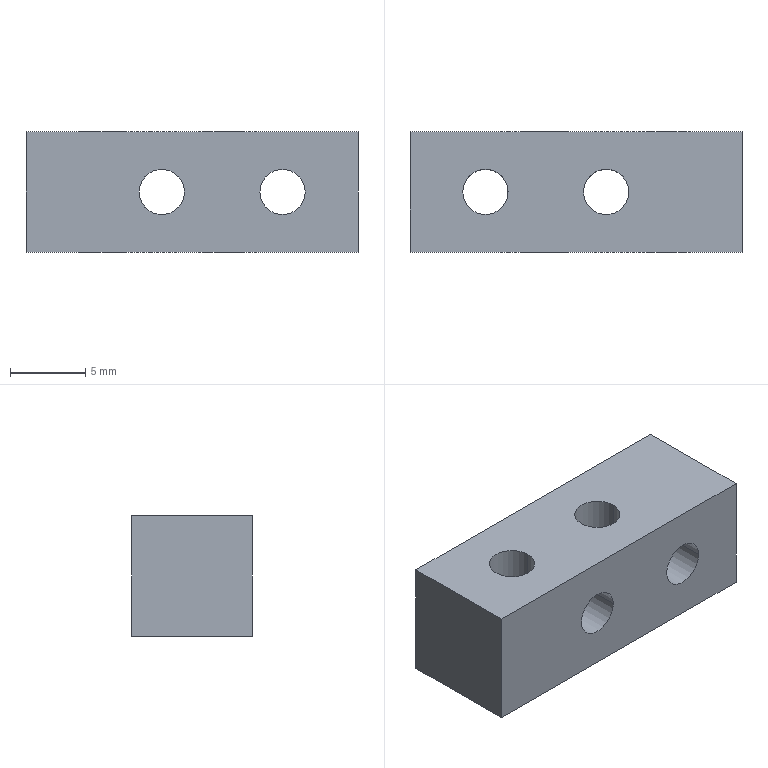Part | SolidWorks | features Extrusion 1, ICE 1 | 1 solid | 14 faces | box 22 x 8 x 8 mm | volume 1182 mm3 | cylinder 8 | plane 6 | commonest cylinder face diameters 3 x8
STEP:
#1=CARTESIAN_POINT('',(7.5,-4.,4.));
#2=VERTEX_POINT('',#1);
#3=CARTESIAN_POINT('',(4.5,-4.,4.));
#4=VERTEX_POINT('',#3);
#5=CARTESIAN_POINT('',(6.,-4.,4.));
#6=DIRECTION('',(0.,1.,0.));
#7=DIRECTION('',(-1.,0.,0.));
#8=AXIS2_PLACEMENT_3D('',#5,#6,#7);
#9=CIRCLE('',#8,1.5);
#10=EDGE_CURVE('',#2,#4,#9,.T.);
#11=ORIENTED_EDGE('',*,*,#10,.F.);
#12=CARTESIAN_POINT('',(7.5,4.,4.));
#13=VERTEX_POINT('',#12);
#14=CARTESIAN_POINT('',(7.5,-4.,4.));
#15=DIRECTION('',(0.,1.,0.));
#16=VECTOR('',#15,1000.);
#17=LINE('',#14,#16);
#18=EDGE_CURVE('',#2,#13,#17,.T.);
#19=ORIENTED_EDGE('',*,*,#18,.T.);
#20=CARTESIAN_POINT('',(4.5,4.,4.));
#21=VERTEX_POINT('',#20);
#22=CARTESIAN_POINT('',(6.,4.,4.));
#23=DIRECTION('',(0.,1.,0.));
#24=DIRECTION('',(-1.,0.,0.));
#25=AXIS2_PLACEMENT_3D('',#22,#23,#24);
#26=CIRCLE('',#25,1.5);
#27=EDGE_CURVE('',#13,#21,#26,.T.);
#28=ORIENTED_EDGE('',*,*,#27,.T.);
#29=CARTESIAN_POINT('',(4.5,-4.,4.));
#30=DIRECTION('',(0.,1.,0.));
#31=VECTOR('',#30,1000.);
#32=LINE('',#29,#31);
#33=EDGE_CURVE('',#4,#21,#32,.T.);
#34=ORIENTED_EDGE('',*,*,#33,.F.);
#35=EDGE_LOOP('',(#11,#19,#28,#34));
#36=FACE_OUTER_BOUND('',#35,.T.);
#37=CARTESIAN_POINT('',(6.,-4.,4.));
#38=DIRECTION('',(0.,1.,0.));
#39=DIRECTION('',(-1.,0.,0.));
#40=AXIS2_PLACEMENT_3D('',#37,#38,#39);
#41=CYLINDRICAL_SURFACE('',#40,1.5);
#42=ADVANCED_FACE('',(#36),#41,.F.);
#43=CARTESIAN_POINT('',(-0.5,-4.,4.));
#44=VERTEX_POINT('',#43);
#45=CARTESIAN_POINT('',(-3.5,-4.,4.));
#46=VERTEX_POINT('',#45);
#47=CARTESIAN_POINT('',(-2.,-4.,4.));
#48=DIRECTION('',(0.,1.,0.));
#49=DIRECTION('',(-1.,0.,0.));
#50=AXIS2_PLACEMENT_3D('',#47,#48,#49);
#51=CIRCLE('',#50,1.5);
#52=EDGE_CURVE('',#44,#46,#51,.T.);
#53=ORIENTED_EDGE('',*,*,#52,.F.);
#54=CARTESIAN_POINT('',(-0.5,4.,4.));
#55=VERTEX_POINT('',#54);
#56=CARTESIAN_POINT('',(-0.5,-4.,4.));
#57=DIRECTION('',(0.,1.,0.));
#58=VECTOR('',#57,1000.);
#59=LINE('',#56,#58);
#60=EDGE_CURVE('',#44,#55,#59,.T.);
#61=ORIENTED_EDGE('',*,*,#60,.T.);
#62=CARTESIAN_POINT('',(-3.5,4.,4.));
#63=VERTEX_POINT('',#62);
#64=CARTESIAN_POINT('',(-2.,4.,4.));
#65=DIRECTION('',(0.,1.,0.));
#66=DIRECTION('',(-1.,0.,0.));
#67=AXIS2_PLACEMENT_3D('',#64,#65,#66);
#68=CIRCLE('',#67,1.5);
#69=EDGE_CURVE('',#55,#63,#68,.T.);
#70=ORIENTED_EDGE('',*,*,#69,.T.);
#71=CARTESIAN_POINT('',(-3.5,-4.,4.));
#72=DIRECTION('',(0.,1.,0.));
#73=VECTOR('',#72,1000.);
#74=LINE('',#71,#73);
#75=EDGE_CURVE('',#46,#63,#74,.T.);
#76=ORIENTED_EDGE('',*,*,#75,.F.);
#77=EDGE_LOOP('',(#53,#61,#70,#76));
#78=FACE_OUTER_BOUND('',#77,.T.);
#79=CARTESIAN_POINT('',(-2.,-4.,4.));
#80=DIRECTION('',(0.,1.,0.));
#81=DIRECTION('',(-1.,0.,0.));
#82=AXIS2_PLACEMENT_3D('',#79,#80,#81);
#83=CYLINDRICAL_SURFACE('',#82,1.5);
#84=ADVANCED_FACE('',(#78),#83,.F.);
#85=CARTESIAN_POINT('',(0.5,0.,8.));
#86=VERTEX_POINT('',#85);
#87=CARTESIAN_POINT('',(3.5,0.,8.));
#88=VERTEX_POINT('',#87);
#89=CARTESIAN_POINT('',(2.,0.,8.));
#90=DIRECTION('',(0.,0.,1.));
#91=DIRECTION('',(1.,0.,0.));
#92=AXIS2_PLACEMENT_3D('',#89,#90,#91);
#93=CIRCLE('',#92,1.5);
#94=EDGE_CURVE('',#86,#88,#93,.T.);
#95=ORIENTED_EDGE('',*,*,#94,.T.);
#96=CARTESIAN_POINT('',(3.5,0.,0.));
#97=VERTEX_POINT('',#96);
#98=CARTESIAN_POINT('',(3.5,0.,8.));
#99=DIRECTION('',(0.,0.,-1.));
#100=VECTOR('',#99,1000.);
#101=LINE('',#98,#100);
#102=EDGE_CURVE('',#88,#97,#101,.T.);
#103=ORIENTED_EDGE('',*,*,#102,.T.);
#104=CARTESIAN_POINT('',(0.5,0.,0.));
#105=VERTEX_POINT('',#104);
#106=CARTESIAN_POINT('',(2.,0.,0.));
#107=DIRECTION('',(0.,0.,1.));
#108=DIRECTION('',(1.,0.,0.));
#109=AXIS2_PLACEMENT_3D('',#106,#107,#108);
#110=CIRCLE('',#109,1.5);
#111=EDGE_CURVE('',#105,#97,#110,.T.);
#112=ORIENTED_EDGE('',*,*,#111,.F.);
#113=CARTESIAN_POINT('',(0.5,0.,8.));
#114=DIRECTION('',(0.,0.,-1.));
#115=VECTOR('',#114,1000.);
#116=LINE('',#113,#115);
#117=EDGE_CURVE('',#86,#105,#116,.T.);
#118=ORIENTED_EDGE('',*,*,#117,.F.);
#119=EDGE_LOOP('',(#95,#103,#112,#118));
#120=FACE_OUTER_BOUND('',#119,.T.);
#121=CARTESIAN_POINT('',(2.,0.,8.));
#122=DIRECTION('',(0.,0.,-1.));
#123=DIRECTION('',(-1.,0.,0.));
#124=AXIS2_PLACEMENT_3D('',#121,#122,#123);
#125=CYLINDRICAL_SURFACE('',#124,1.5);
#126=ADVANCED_FACE('',(#120),#125,.F.);
#127=CARTESIAN_POINT('',(-7.5,0.,8.));
#128=VERTEX_POINT('',#127);
#129=CARTESIAN_POINT('',(-4.5,0.,8.));
#130=VERTEX_POINT('',#129);
#131=CARTESIAN_POINT('',(-6.,0.,8.));
#132=DIRECTION('',(0.,0.,1.));
#133=DIRECTION('',(1.,0.,0.));
#134=AXIS2_PLACEMENT_3D('',#131,#132,#133);
#135=CIRCLE('',#134,1.5);
#136=EDGE_CURVE('',#128,#130,#135,.T.);
#137=ORIENTED_EDGE('',*,*,#136,.T.);
#138=CARTESIAN_POINT('',(-4.5,0.,0.));
#139=VERTEX_POINT('',#138);
#140=CARTESIAN_POINT('',(-4.5,0.,8.));
#141=DIRECTION('',(0.,0.,-1.));
#142=VECTOR('',#141,1000.);
#143=LINE('',#140,#142);
#144=EDGE_CURVE('',#130,#139,#143,.T.);
#145=ORIENTED_EDGE('',*,*,#144,.T.);
#146=CARTESIAN_POINT('',(-7.5,0.,0.));
#147=VERTEX_POINT('',#146);
#148=CARTESIAN_POINT('',(-6.,0.,0.));
#149=DIRECTION('',(0.,0.,1.));
#150=DIRECTION('',(1.,0.,0.));
#151=AXIS2_PLACEMENT_3D('',#148,#149,#150);
#152=CIRCLE('',#151,1.5);
#153=EDGE_CURVE('',#147,#139,#152,.T.);
#154=ORIENTED_EDGE('',*,*,#153,.F.);
#155=CARTESIAN_POINT('',(-7.5,0.,8.));
#156=DIRECTION('',(0.,0.,-1.));
#157=VECTOR('',#156,1000.);
#158=LINE('',#155,#157);
#159=EDGE_CURVE('',#128,#147,#158,.T.);
#160=ORIENTED_EDGE('',*,*,#159,.F.);
#161=EDGE_LOOP('',(#137,#145,#154,#160));
#162=FACE_OUTER_BOUND('',#161,.T.);
#163=CARTESIAN_POINT('',(-6.,0.,8.));
#164=DIRECTION('',(0.,0.,-1.));
#165=DIRECTION('',(-1.,0.,0.));
#166=AXIS2_PLACEMENT_3D('',#163,#164,#165);
#167=CYLINDRICAL_SURFACE('',#166,1.5);
#168=ADVANCED_FACE('',(#162),#167,.F.);
#169=CARTESIAN_POINT('',(-11.,4.,8.));
#170=VERTEX_POINT('',#169);
#171=CARTESIAN_POINT('',(-11.,-4.,8.));
#172=VERTEX_POINT('',#171);
#173=CARTESIAN_POINT('',(-11.,4.,8.));
#174=DIRECTION('',(0.,-1.,0.));
#175=VECTOR('',#174,1000.);
#176=LINE('',#173,#175);
#177=EDGE_CURVE('',#170,#172,#176,.T.);
#178=ORIENTED_EDGE('',*,*,#177,.T.);
#179=CARTESIAN_POINT('',(11.,-4.,8.));
#180=VERTEX_POINT('',#179);
#181=CARTESIAN_POINT('',(11.,-4.,8.));
#182=DIRECTION('',(1.,0.,0.));
#183=VECTOR('',#182,1000.);
#184=LINE('',#181,#183);
#185=EDGE_CURVE('',#172,#180,#184,.T.);
#186=ORIENTED_EDGE('',*,*,#185,.T.);
#187=CARTESIAN_POINT('',(11.,4.,8.));
#188=VERTEX_POINT('',#187);
#189=CARTESIAN_POINT('',(11.,4.,8.));
#190=DIRECTION('',(0.,1.,0.));
#191=VECTOR('',#190,1000.);
#192=LINE('',#189,#191);
#193=EDGE_CURVE('',#180,#188,#192,.T.);
#194=ORIENTED_EDGE('',*,*,#193,.T.);
#195=CARTESIAN_POINT('',(11.,4.,8.));
#196=DIRECTION('',(-1.,0.,0.));
#197=VECTOR('',#196,1000.);
#198=LINE('',#195,#197);
#199=EDGE_CURVE('',#188,#170,#198,.T.);
#200=ORIENTED_EDGE('',*,*,#199,.T.);
#201=EDGE_LOOP('',(#178,#186,#194,#200));
#202=FACE_OUTER_BOUND('',#201,.T.);
#203=ORIENTED_EDGE('',*,*,#136,.F.);
#204=CARTESIAN_POINT('',(-6.,0.,8.));
#205=DIRECTION('',(0.,0.,1.));
#206=DIRECTION('',(1.,0.,0.));
#207=AXIS2_PLACEMENT_3D('',#204,#205,#206);
#208=CIRCLE('',#207,1.5);
#209=EDGE_CURVE('',#130,#128,#208,.T.);
#210=ORIENTED_EDGE('',*,*,#209,.F.);
#211=EDGE_LOOP('',(#203,#210));
#212=FACE_BOUND('',#211,.T.);
#213=ORIENTED_EDGE('',*,*,#94,.F.);
#214=CARTESIAN_POINT('',(2.,0.,8.));
#215=DIRECTION('',(0.,0.,1.));
#216=DIRECTION('',(1.,0.,0.));
#217=AXIS2_PLACEMENT_3D('',#214,#215,#216);
#218=CIRCLE('',#217,1.5);
#219=EDGE_CURVE('',#88,#86,#218,.T.);
#220=ORIENTED_EDGE('',*,*,#219,.F.);
#221=EDGE_LOOP('',(#213,#220));
#222=FACE_BOUND('',#221,.T.);
#223=CARTESIAN_POINT('',(0.,0.,8.));
#224=DIRECTION('',(0.,0.,-1.));
#225=DIRECTION('',(-1.,0.,0.));
#226=AXIS2_PLACEMENT_3D('',#223,#224,#225);
#227=PLANE('',#226);
#228=ADVANCED_FACE('',(#202,#212,#222),#227,.F.);
#229=ORIENTED_EDGE('',*,*,#153,.T.);
#230=CARTESIAN_POINT('',(-6.,0.,0.));
#231=DIRECTION('',(0.,0.,1.));
#232=DIRECTION('',(1.,0.,0.));
#233=AXIS2_PLACEMENT_3D('',#230,#231,#232);
#234=CIRCLE('',#233,1.5);
#235=EDGE_CURVE('',#139,#147,#234,.T.);
#236=ORIENTED_EDGE('',*,*,#235,.T.);
#237=EDGE_LOOP('',(#229,#236));
#238=FACE_BOUND('',#237,.T.);
#239=CARTESIAN_POINT('',(-11.,4.,0.));
#240=VERTEX_POINT('',#239);
#241=CARTESIAN_POINT('',(-11.,-4.,0.));
#242=VERTEX_POINT('',#241);
#243=CARTESIAN_POINT('',(-11.,4.,0.));
#244=DIRECTION('',(0.,-1.,0.));
#245=VECTOR('',#244,1000.);
#246=LINE('',#243,#245);
#247=EDGE_CURVE('',#240,#242,#246,.T.);
#248=ORIENTED_EDGE('',*,*,#247,.F.);
#249=CARTESIAN_POINT('',(11.,4.,0.));
#250=VERTEX_POINT('',#249);
#251=CARTESIAN_POINT('',(11.,4.,0.));
#252=DIRECTION('',(-1.,0.,0.));
#253=VECTOR('',#252,1000.);
#254=LINE('',#251,#253);
#255=EDGE_CURVE('',#250,#240,#254,.T.);
#256=ORIENTED_EDGE('',*,*,#255,.F.);
#257=CARTESIAN_POINT('',(11.,-4.,0.));
#258=VERTEX_POINT('',#257);
#259=CARTESIAN_POINT('',(11.,4.,0.));
#260=DIRECTION('',(0.,1.,0.));
#261=VECTOR('',#260,1000.);
#262=LINE('',#259,#261);
#263=EDGE_CURVE('',#258,#250,#262,.T.);
#264=ORIENTED_EDGE('',*,*,#263,.F.);
#265=CARTESIAN_POINT('',(11.,-4.,0.));
#266=DIRECTION('',(1.,0.,0.));
#267=VECTOR('',#266,1000.);
#268=LINE('',#265,#267);
#269=EDGE_CURVE('',#242,#258,#268,.T.);
#270=ORIENTED_EDGE('',*,*,#269,.F.);
#271=EDGE_LOOP('',(#248,#256,#264,#270));
#272=FACE_OUTER_BOUND('',#271,.T.);
#273=ORIENTED_EDGE('',*,*,#111,.T.);
#274=CARTESIAN_POINT('',(2.,0.,0.));
#275=DIRECTION('',(0.,0.,1.));
#276=DIRECTION('',(1.,0.,0.));
#277=AXIS2_PLACEMENT_3D('',#274,#275,#276);
#278=CIRCLE('',#277,1.5);
#279=EDGE_CURVE('',#97,#105,#278,.T.);
#280=ORIENTED_EDGE('',*,*,#279,.T.);
#281=EDGE_LOOP('',(#273,#280));
#282=FACE_BOUND('',#281,.T.);
#283=CARTESIAN_POINT('',(0.,0.,0.));
#284=DIRECTION('',(0.,0.,-1.));
#285=DIRECTION('',(-1.,0.,0.));
#286=AXIS2_PLACEMENT_3D('',#283,#284,#285);
#287=PLANE('',#286);
#288=ADVANCED_FACE('',(#238,#272,#282),#287,.T.);
#289=ORIENTED_EDGE('',*,*,#247,.T.);
#290=CARTESIAN_POINT('',(-11.,-4.,8.));
#291=DIRECTION('',(0.,0.,-1.));
#292=VECTOR('',#291,1000.);
#293=LINE('',#290,#292);
#294=EDGE_CURVE('',#172,#242,#293,.T.);
#295=ORIENTED_EDGE('',*,*,#294,.F.);
#296=ORIENTED_EDGE('',*,*,#177,.F.);
#297=CARTESIAN_POINT('',(-11.,4.,8.));
#298=DIRECTION('',(0.,0.,-1.));
#299=VECTOR('',#298,1000.);
#300=LINE('',#297,#299);
#301=EDGE_CURVE('',#170,#240,#300,.T.);
#302=ORIENTED_EDGE('',*,*,#301,.T.);
#303=EDGE_LOOP('',(#289,#295,#296,#302));
#304=FACE_OUTER_BOUND('',#303,.T.);
#305=CARTESIAN_POINT('',(-11.,4.,8.));
#306=DIRECTION('',(1.,0.,0.));
#307=DIRECTION('',(0.,1.,0.));
#308=AXIS2_PLACEMENT_3D('',#305,#306,#307);
#309=PLANE('',#308);
#310=ADVANCED_FACE('',(#304),#309,.F.);
#311=CARTESIAN_POINT('',(6.,-4.,4.));
#312=DIRECTION('',(0.,1.,0.));
#313=DIRECTION('',(-1.,0.,0.));
#314=AXIS2_PLACEMENT_3D('',#311,#312,#313);
#315=CIRCLE('',#314,1.5);
#316=EDGE_CURVE('',#4,#2,#315,.T.);
#317=ORIENTED_EDGE('',*,*,#316,.T.);
#318=ORIENTED_EDGE('',*,*,#10,.T.);
#319=EDGE_LOOP('',(#317,#318));
#320=FACE_BOUND('',#319,.T.);
#321=CARTESIAN_POINT('',(-2.,-4.,4.));
#322=DIRECTION('',(0.,1.,0.));
#323=DIRECTION('',(-1.,0.,0.));
#324=AXIS2_PLACEMENT_3D('',#321,#322,#323);
#325=CIRCLE('',#324,1.5);
#326=EDGE_CURVE('',#46,#44,#325,.T.);
#327=ORIENTED_EDGE('',*,*,#326,.T.);
#328=ORIENTED_EDGE('',*,*,#52,.T.);
#329=EDGE_LOOP('',(#327,#328));
#330=FACE_BOUND('',#329,.T.);
#331=ORIENTED_EDGE('',*,*,#269,.T.);
#332=CARTESIAN_POINT('',(11.,-4.,8.));
#333=DIRECTION('',(0.,0.,-1.));
#334=VECTOR('',#333,1000.);
#335=LINE('',#332,#334);
#336=EDGE_CURVE('',#180,#258,#335,.T.);
#337=ORIENTED_EDGE('',*,*,#336,.F.);
#338=ORIENTED_EDGE('',*,*,#185,.F.);
#339=ORIENTED_EDGE('',*,*,#294,.T.);
#340=EDGE_LOOP('',(#331,#337,#338,#339));
#341=FACE_OUTER_BOUND('',#340,.T.);
#342=CARTESIAN_POINT('',(11.,-4.,8.));
#343=DIRECTION('',(0.,1.,0.));
#344=DIRECTION('',(-1.,0.,0.));
#345=AXIS2_PLACEMENT_3D('',#342,#343,#344);
#346=PLANE('',#345);
#347=ADVANCED_FACE('',(#320,#330,#341),#346,.F.);
#348=ORIENTED_EDGE('',*,*,#263,.T.);
#349=CARTESIAN_POINT('',(11.,4.,8.));
#350=DIRECTION('',(0.,0.,-1.));
#351=VECTOR('',#350,1000.);
#352=LINE('',#349,#351);
#353=EDGE_CURVE('',#188,#250,#352,.T.);
#354=ORIENTED_EDGE('',*,*,#353,.F.);
#355=ORIENTED_EDGE('',*,*,#193,.F.);
#356=ORIENTED_EDGE('',*,*,#336,.T.);
#357=EDGE_LOOP('',(#348,#354,#355,#356));
#358=FACE_OUTER_BOUND('',#357,.T.);
#359=CARTESIAN_POINT('',(11.,4.,8.));
#360=DIRECTION('',(-1.,0.,0.));
#361=DIRECTION('',(0.,-1.,0.));
#362=AXIS2_PLACEMENT_3D('',#359,#360,#361);
#363=PLANE('',#362);
#364=ADVANCED_FACE('',(#358),#363,.F.);
#365=CARTESIAN_POINT('',(6.,4.,4.));
#366=DIRECTION('',(0.,1.,0.));
#367=DIRECTION('',(-1.,0.,0.));
#368=AXIS2_PLACEMENT_3D('',#365,#366,#367);
#369=CIRCLE('',#368,1.5);
#370=EDGE_CURVE('',#21,#13,#369,.T.);
#371=ORIENTED_EDGE('',*,*,#370,.F.);
#372=ORIENTED_EDGE('',*,*,#27,.F.);
#373=EDGE_LOOP('',(#371,#372));
#374=FACE_BOUND('',#373,.T.);
#375=CARTESIAN_POINT('',(-2.,4.,4.));
#376=DIRECTION('',(0.,1.,0.));
#377=DIRECTION('',(-1.,0.,0.));
#378=AXIS2_PLACEMENT_3D('',#375,#376,#377);
#379=CIRCLE('',#378,1.5);
#380=EDGE_CURVE('',#63,#55,#379,.T.);
#381=ORIENTED_EDGE('',*,*,#380,.F.);
#382=ORIENTED_EDGE('',*,*,#69,.F.);
#383=EDGE_LOOP('',(#381,#382));
#384=FACE_BOUND('',#383,.T.);
#385=ORIENTED_EDGE('',*,*,#255,.T.);
#386=ORIENTED_EDGE('',*,*,#301,.F.);
#387=ORIENTED_EDGE('',*,*,#199,.F.);
#388=ORIENTED_EDGE('',*,*,#353,.T.);
#389=EDGE_LOOP('',(#385,#386,#387,#388));
#390=FACE_OUTER_BOUND('',#389,.T.);
#391=CARTESIAN_POINT('',(11.,4.,8.));
#392=DIRECTION('',(0.,-1.,0.));
#393=DIRECTION('',(1.,0.,0.));
#394=AXIS2_PLACEMENT_3D('',#391,#392,#393);
#395=PLANE('',#394);
#396=ADVANCED_FACE('',(#374,#384,#390),#395,.F.);
#397=ORIENTED_EDGE('',*,*,#144,.F.);
#398=ORIENTED_EDGE('',*,*,#209,.T.);
#399=ORIENTED_EDGE('',*,*,#159,.T.);
#400=ORIENTED_EDGE('',*,*,#235,.F.);
#401=EDGE_LOOP('',(#397,#398,#399,#400));
#402=FACE_OUTER_BOUND('',#401,.T.);
#403=CARTESIAN_POINT('',(-6.,0.,8.));
#404=DIRECTION('',(0.,0.,-1.));
#405=DIRECTION('',(-1.,0.,0.));
#406=AXIS2_PLACEMENT_3D('',#403,#404,#405);
#407=CYLINDRICAL_SURFACE('',#406,1.5);
#408=ADVANCED_FACE('',(#402),#407,.F.);
#409=ORIENTED_EDGE('',*,*,#102,.F.);
#410=ORIENTED_EDGE('',*,*,#219,.T.);
#411=ORIENTED_EDGE('',*,*,#117,.T.);
#412=ORIENTED_EDGE('',*,*,#279,.F.);
#413=EDGE_LOOP('',(#409,#410,#411,#412));
#414=FACE_OUTER_BOUND('',#413,.T.);
#415=CARTESIAN_POINT('',(2.,0.,8.));
#416=DIRECTION('',(0.,0.,-1.));
#417=DIRECTION('',(-1.,0.,0.));
#418=AXIS2_PLACEMENT_3D('',#415,#416,#417);
#419=CYLINDRICAL_SURFACE('',#418,1.5);
#420=ADVANCED_FACE('',(#414),#419,.F.);
#421=ORIENTED_EDGE('',*,*,#60,.F.);
#422=ORIENTED_EDGE('',*,*,#326,.F.);
#423=ORIENTED_EDGE('',*,*,#75,.T.);
#424=ORIENTED_EDGE('',*,*,#380,.T.);
#425=EDGE_LOOP('',(#421,#422,#423,#424));
#426=FACE_OUTER_BOUND('',#425,.T.);
#427=CARTESIAN_POINT('',(-2.,-4.,4.));
#428=DIRECTION('',(0.,1.,0.));
#429=DIRECTION('',(-1.,0.,0.));
#430=AXIS2_PLACEMENT_3D('',#427,#428,#429);
#431=CYLINDRICAL_SURFACE('',#430,1.5);
#432=ADVANCED_FACE('',(#426),#431,.F.);
#433=ORIENTED_EDGE('',*,*,#18,.F.);
#434=ORIENTED_EDGE('',*,*,#316,.F.);
#435=ORIENTED_EDGE('',*,*,#33,.T.);
#436=ORIENTED_EDGE('',*,*,#370,.T.);
#437=EDGE_LOOP('',(#433,#434,#435,#436));
#438=FACE_OUTER_BOUND('',#437,.T.);
#439=CARTESIAN_POINT('',(6.,-4.,4.));
#440=DIRECTION('',(0.,1.,0.));
#441=DIRECTION('',(-1.,0.,0.));
#442=AXIS2_PLACEMENT_3D('',#439,#440,#441);
#443=CYLINDRICAL_SURFACE('',#442,1.5);
#444=ADVANCED_FACE('',(#438),#443,.F.);
#445=CLOSED_SHELL('',(#42,#84,#126,#168,#228,#288,#310,#347,#364,#396,#408,#420,#432,#444));
#446=MANIFOLD_SOLID_BREP('',#445);
#447=CARTESIAN_POINT('',(0.,0.,0.));
#448=DIRECTION('',(0.,0.,1.));
#449=DIRECTION('',(1.,0.,0.));
#450=AXIS2_PLACEMENT_3D('',#447,#448,#449);
#451=(LENGTH_UNIT()NAMED_UNIT(*)SI_UNIT(.MILLI.,.METRE.));
#452=UNCERTAINTY_MEASURE_WITH_UNIT(LENGTH_MEASURE(0.00001),#451,'','');
#453=(NAMED_UNIT(*)PLANE_ANGLE_UNIT()SI_UNIT($,.RADIAN.));
#454=(NAMED_UNIT(*)SI_UNIT($,.STERADIAN.)SOLID_ANGLE_UNIT());
#455=(GEOMETRIC_REPRESENTATION_CONTEXT(3)GLOBAL_UNCERTAINTY_ASSIGNED_CONTEXT((#452))GLOBAL_UNIT_ASSIGNED_CONTEXT((#451,#453,#454))REPRESENTATION_CONTEXT('',''));
#456=ADVANCED_BREP_SHAPE_REPRESENTATION('',(#446,#450),#455);